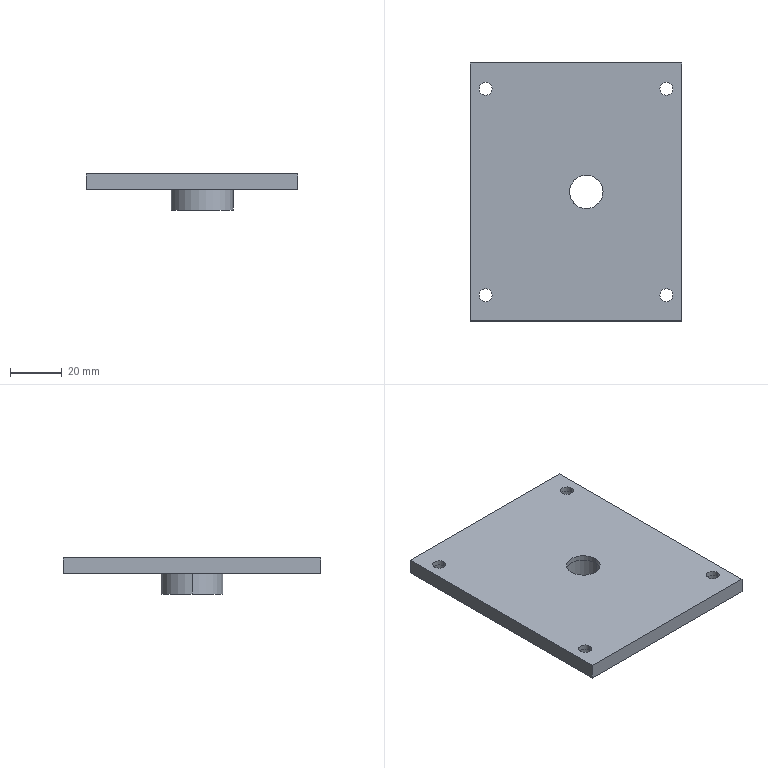Part | SolidWorks | features ICE 5, Extrusion 1 | 1 solid | 34 faces | box 82 x 100 x 14 mm | volume 49472 mm3 | cylinder 22 | plane 12 | commonest cylinder face diameters 5 x8 8 x8 13 x2 15 x2 24 x2
STEP:
#1=CARTESIAN_POINT('',(37.5,40.,6.));
#2=VERTEX_POINT('',#1);
#3=CARTESIAN_POINT('',(32.5,40.,6.));
#4=VERTEX_POINT('',#3);
#5=CARTESIAN_POINT('',(35.,40.,6.));
#6=DIRECTION('',(0.,0.,-1.));
#7=DIRECTION('',(1.,0.,0.));
#8=AXIS2_PLACEMENT_3D('',#5,#6,#7);
#9=CIRCLE('',#8,2.5);
#10=EDGE_CURVE('',#2,#4,#9,.T.);
#11=ORIENTED_EDGE('',*,*,#10,.F.);
#12=CARTESIAN_POINT('',(37.5,40.,4.));
#13=VERTEX_POINT('',#12);
#14=CARTESIAN_POINT('',(37.5,40.,6.));
#15=DIRECTION('',(0.,0.,-1.));
#16=VECTOR('',#15,1000.);
#17=LINE('',#14,#16);
#18=EDGE_CURVE('',#2,#13,#17,.T.);
#19=ORIENTED_EDGE('',*,*,#18,.T.);
#20=CARTESIAN_POINT('',(32.5,40.,4.));
#21=VERTEX_POINT('',#20);
#22=CARTESIAN_POINT('',(35.,40.,4.));
#23=DIRECTION('',(0.,0.,-1.));
#24=DIRECTION('',(-1.,0.,0.));
#25=AXIS2_PLACEMENT_3D('',#22,#23,#24);
#26=CIRCLE('',#25,2.5);
#27=EDGE_CURVE('',#13,#21,#26,.T.);
#28=ORIENTED_EDGE('',*,*,#27,.T.);
#29=CARTESIAN_POINT('',(32.5,40.,6.));
#30=DIRECTION('',(0.,0.,-1.));
#31=VECTOR('',#30,1000.);
#32=LINE('',#29,#31);
#33=EDGE_CURVE('',#4,#21,#32,.T.);
#34=ORIENTED_EDGE('',*,*,#33,.F.);
#35=EDGE_LOOP('',(#11,#19,#28,#34));
#36=FACE_OUTER_BOUND('',#35,.T.);
#37=CARTESIAN_POINT('',(35.,40.,6.));
#38=DIRECTION('',(0.,0.,-1.));
#39=DIRECTION('',(-1.,0.,0.));
#40=AXIS2_PLACEMENT_3D('',#37,#38,#39);
#41=CYLINDRICAL_SURFACE('',#40,2.5);
#42=ADVANCED_FACE('',(#36),#41,.F.);
#43=CARTESIAN_POINT('',(37.5,-40.,6.));
#44=VERTEX_POINT('',#43);
#45=CARTESIAN_POINT('',(32.5,-40.,6.));
#46=VERTEX_POINT('',#45);
#47=CARTESIAN_POINT('',(35.,-40.,6.));
#48=DIRECTION('',(0.,0.,-1.));
#49=DIRECTION('',(-1.,0.,0.));
#50=AXIS2_PLACEMENT_3D('',#47,#48,#49);
#51=CIRCLE('',#50,2.5);
#52=EDGE_CURVE('',#44,#46,#51,.T.);
#53=ORIENTED_EDGE('',*,*,#52,.F.);
#54=CARTESIAN_POINT('',(37.5,-40.,4.));
#55=VERTEX_POINT('',#54);
#56=CARTESIAN_POINT('',(37.5,-40.,6.));
#57=DIRECTION('',(0.,0.,-1.));
#58=VECTOR('',#57,1000.);
#59=LINE('',#56,#58);
#60=EDGE_CURVE('',#44,#55,#59,.T.);
#61=ORIENTED_EDGE('',*,*,#60,.T.);
#62=CARTESIAN_POINT('',(32.5,-40.,4.));
#63=VERTEX_POINT('',#62);
#64=CARTESIAN_POINT('',(35.,-40.,4.));
#65=DIRECTION('',(0.,0.,1.));
#66=DIRECTION('',(1.,0.,0.));
#67=AXIS2_PLACEMENT_3D('',#64,#65,#66);
#68=CIRCLE('',#67,2.5);
#69=EDGE_CURVE('',#63,#55,#68,.T.);
#70=ORIENTED_EDGE('',*,*,#69,.F.);
#71=CARTESIAN_POINT('',(32.5,-40.,6.));
#72=DIRECTION('',(0.,0.,-1.));
#73=VECTOR('',#72,1000.);
#74=LINE('',#71,#73);
#75=EDGE_CURVE('',#46,#63,#74,.T.);
#76=ORIENTED_EDGE('',*,*,#75,.F.);
#77=EDGE_LOOP('',(#53,#61,#70,#76));
#78=FACE_OUTER_BOUND('',#77,.T.);
#79=CARTESIAN_POINT('',(35.,-40.,6.));
#80=DIRECTION('',(0.,0.,-1.));
#81=DIRECTION('',(-1.,0.,0.));
#82=AXIS2_PLACEMENT_3D('',#79,#80,#81);
#83=CYLINDRICAL_SURFACE('',#82,2.5);
#84=ADVANCED_FACE('',(#78),#83,.F.);
#85=CARTESIAN_POINT('',(-32.5,-40.,6.));
#86=VERTEX_POINT('',#85);
#87=CARTESIAN_POINT('',(-37.5,-40.,6.));
#88=VERTEX_POINT('',#87);
#89=CARTESIAN_POINT('',(-35.,-40.,6.));
#90=DIRECTION('',(0.,0.,-1.));
#91=DIRECTION('',(1.,0.,0.));
#92=AXIS2_PLACEMENT_3D('',#89,#90,#91);
#93=CIRCLE('',#92,2.5);
#94=EDGE_CURVE('',#86,#88,#93,.T.);
#95=ORIENTED_EDGE('',*,*,#94,.F.);
#96=CARTESIAN_POINT('',(-32.5,-40.,4.));
#97=VERTEX_POINT('',#96);
#98=CARTESIAN_POINT('',(-32.5,-40.,6.));
#99=DIRECTION('',(0.,0.,-1.));
#100=VECTOR('',#99,1000.);
#101=LINE('',#98,#100);
#102=EDGE_CURVE('',#86,#97,#101,.T.);
#103=ORIENTED_EDGE('',*,*,#102,.T.);
#104=CARTESIAN_POINT('',(-37.5,-40.,4.));
#105=VERTEX_POINT('',#104);
#106=CARTESIAN_POINT('',(-35.,-40.,4.));
#107=DIRECTION('',(0.,0.,-1.));
#108=DIRECTION('',(-1.,0.,0.));
#109=AXIS2_PLACEMENT_3D('',#106,#107,#108);
#110=CIRCLE('',#109,2.5);
#111=EDGE_CURVE('',#97,#105,#110,.T.);
#112=ORIENTED_EDGE('',*,*,#111,.T.);
#113=CARTESIAN_POINT('',(-37.5,-40.,6.));
#114=DIRECTION('',(0.,0.,-1.));
#115=VECTOR('',#114,1000.);
#116=LINE('',#113,#115);
#117=EDGE_CURVE('',#88,#105,#116,.T.);
#118=ORIENTED_EDGE('',*,*,#117,.F.);
#119=EDGE_LOOP('',(#95,#103,#112,#118));
#120=FACE_OUTER_BOUND('',#119,.T.);
#121=CARTESIAN_POINT('',(-35.,-40.,6.));
#122=DIRECTION('',(0.,0.,-1.));
#123=DIRECTION('',(-1.,0.,0.));
#124=AXIS2_PLACEMENT_3D('',#121,#122,#123);
#125=CYLINDRICAL_SURFACE('',#124,2.5);
#126=ADVANCED_FACE('',(#120),#125,.F.);
#127=CARTESIAN_POINT('',(-32.5,40.,6.));
#128=VERTEX_POINT('',#127);
#129=CARTESIAN_POINT('',(-37.5,40.,6.));
#130=VERTEX_POINT('',#129);
#131=CARTESIAN_POINT('',(-35.,40.,6.));
#132=DIRECTION('',(0.,0.,-1.));
#133=DIRECTION('',(-1.,0.,0.));
#134=AXIS2_PLACEMENT_3D('',#131,#132,#133);
#135=CIRCLE('',#134,2.5);
#136=EDGE_CURVE('',#128,#130,#135,.T.);
#137=ORIENTED_EDGE('',*,*,#136,.F.);
#138=CARTESIAN_POINT('',(-32.5,40.,4.));
#139=VERTEX_POINT('',#138);
#140=CARTESIAN_POINT('',(-32.5,40.,6.));
#141=DIRECTION('',(0.,0.,-1.));
#142=VECTOR('',#141,1000.);
#143=LINE('',#140,#142);
#144=EDGE_CURVE('',#128,#139,#143,.T.);
#145=ORIENTED_EDGE('',*,*,#144,.T.);
#146=CARTESIAN_POINT('',(-37.5,40.,4.));
#147=VERTEX_POINT('',#146);
#148=CARTESIAN_POINT('',(-35.,40.,4.));
#149=DIRECTION('',(0.,0.,1.));
#150=DIRECTION('',(1.,0.,0.));
#151=AXIS2_PLACEMENT_3D('',#148,#149,#150);
#152=CIRCLE('',#151,2.5);
#153=EDGE_CURVE('',#147,#139,#152,.T.);
#154=ORIENTED_EDGE('',*,*,#153,.F.);
#155=CARTESIAN_POINT('',(-37.5,40.,6.));
#156=DIRECTION('',(0.,0.,-1.));
#157=VECTOR('',#156,1000.);
#158=LINE('',#155,#157);
#159=EDGE_CURVE('',#130,#147,#158,.T.);
#160=ORIENTED_EDGE('',*,*,#159,.F.);
#161=EDGE_LOOP('',(#137,#145,#154,#160));
#162=FACE_OUTER_BOUND('',#161,.T.);
#163=CARTESIAN_POINT('',(-35.,40.,6.));
#164=DIRECTION('',(0.,0.,-1.));
#165=DIRECTION('',(-1.,0.,0.));
#166=AXIS2_PLACEMENT_3D('',#163,#164,#165);
#167=CYLINDRICAL_SURFACE('',#166,2.5);
#168=ADVANCED_FACE('',(#162),#167,.F.);
#169=CARTESIAN_POINT('',(11.5,0.,4.));
#170=VERTEX_POINT('',#169);
#171=CARTESIAN_POINT('',(-3.5,0.,4.));
#172=VERTEX_POINT('',#171);
#173=CARTESIAN_POINT('',(4.,0.,4.));
#174=DIRECTION('',(0.,0.,-1.));
#175=DIRECTION('',(-1.,0.,0.));
#176=AXIS2_PLACEMENT_3D('',#173,#174,#175);
#177=CIRCLE('',#176,7.5);
#178=EDGE_CURVE('',#170,#172,#177,.T.);
#179=ORIENTED_EDGE('',*,*,#178,.F.);
#180=CARTESIAN_POINT('',(11.5,0.,-8.));
#181=VERTEX_POINT('',#180);
#182=CARTESIAN_POINT('',(11.5,0.,4.));
#183=DIRECTION('',(0.,0.,-1.));
#184=VECTOR('',#183,1000.);
#185=LINE('',#182,#184);
#186=EDGE_CURVE('',#170,#181,#185,.T.);
#187=ORIENTED_EDGE('',*,*,#186,.T.);
#188=CARTESIAN_POINT('',(-3.5,0.,-8.));
#189=VERTEX_POINT('',#188);
#190=CARTESIAN_POINT('',(4.,0.,-8.));
#191=DIRECTION('',(0.,0.,-1.));
#192=DIRECTION('',(-1.,0.,0.));
#193=AXIS2_PLACEMENT_3D('',#190,#191,#192);
#194=CIRCLE('',#193,7.5);
#195=EDGE_CURVE('',#181,#189,#194,.T.);
#196=ORIENTED_EDGE('',*,*,#195,.T.);
#197=CARTESIAN_POINT('',(-3.5,0.,4.));
#198=DIRECTION('',(0.,0.,-1.));
#199=VECTOR('',#198,1000.);
#200=LINE('',#197,#199);
#201=EDGE_CURVE('',#172,#189,#200,.T.);
#202=ORIENTED_EDGE('',*,*,#201,.F.);
#203=EDGE_LOOP('',(#179,#187,#196,#202));
#204=FACE_OUTER_BOUND('',#203,.T.);
#205=CARTESIAN_POINT('',(4.,0.,4.));
#206=DIRECTION('',(0.,0.,-1.));
#207=DIRECTION('',(-1.,0.,0.));
#208=AXIS2_PLACEMENT_3D('',#205,#206,#207);
#209=CYLINDRICAL_SURFACE('',#208,7.5);
#210=ADVANCED_FACE('',(#204),#209,.F.);
#211=CARTESIAN_POINT('',(-2.5,0.,4.));
#212=VERTEX_POINT('',#211);
#213=CARTESIAN_POINT('',(10.5,0.,4.));
#214=VERTEX_POINT('',#213);
#215=CARTESIAN_POINT('',(4.,0.,4.));
#216=DIRECTION('',(0.,0.,1.));
#217=DIRECTION('',(1.,0.,0.));
#218=AXIS2_PLACEMENT_3D('',#215,#216,#217);
#219=CIRCLE('',#218,6.5);
#220=EDGE_CURVE('',#212,#214,#219,.T.);
#221=ORIENTED_EDGE('',*,*,#220,.F.);
#222=CARTESIAN_POINT('',(-2.5,0.,6.));
#223=VERTEX_POINT('',#222);
#224=CARTESIAN_POINT('',(-2.5,0.,4.));
#225=DIRECTION('',(0.,0.,1.));
#226=VECTOR('',#225,1000.);
#227=LINE('',#224,#226);
#228=EDGE_CURVE('',#212,#223,#227,.T.);
#229=ORIENTED_EDGE('',*,*,#228,.T.);
#230=CARTESIAN_POINT('',(10.5,0.,6.));
#231=VERTEX_POINT('',#230);
#232=CARTESIAN_POINT('',(4.,0.,6.));
#233=DIRECTION('',(0.,0.,1.));
#234=DIRECTION('',(1.,0.,0.));
#235=AXIS2_PLACEMENT_3D('',#232,#233,#234);
#236=CIRCLE('',#235,6.5);
#237=EDGE_CURVE('',#223,#231,#236,.T.);
#238=ORIENTED_EDGE('',*,*,#237,.T.);
#239=CARTESIAN_POINT('',(10.5,0.,4.));
#240=DIRECTION('',(0.,0.,1.));
#241=VECTOR('',#240,1000.);
#242=LINE('',#239,#241);
#243=EDGE_CURVE('',#214,#231,#242,.T.);
#244=ORIENTED_EDGE('',*,*,#243,.F.);
#245=EDGE_LOOP('',(#221,#229,#238,#244));
#246=FACE_OUTER_BOUND('',#245,.T.);
#247=CARTESIAN_POINT('',(4.,0.,4.));
#248=DIRECTION('',(0.,0.,1.));
#249=DIRECTION('',(1.,0.,0.));
#250=AXIS2_PLACEMENT_3D('',#247,#248,#249);
#251=CYLINDRICAL_SURFACE('',#250,6.5);
#252=ADVANCED_FACE('',(#246),#251,.F.);
#253=CARTESIAN_POINT('',(-31.,40.,4.));
#254=VERTEX_POINT('',#253);
#255=CARTESIAN_POINT('',(-39.,40.,4.));
#256=VERTEX_POINT('',#255);
#257=CARTESIAN_POINT('',(-35.,40.,4.));
#258=DIRECTION('',(0.,0.,-1.));
#259=DIRECTION('',(1.,0.,0.));
#260=AXIS2_PLACEMENT_3D('',#257,#258,#259);
#261=CIRCLE('',#260,4.);
#262=EDGE_CURVE('',#254,#256,#261,.T.);
#263=ORIENTED_EDGE('',*,*,#262,.F.);
#264=CARTESIAN_POINT('',(-31.,40.,0.));
#265=VERTEX_POINT('',#264);
#266=CARTESIAN_POINT('',(-31.,40.,4.));
#267=DIRECTION('',(0.,0.,-1.));
#268=VECTOR('',#267,1000.);
#269=LINE('',#266,#268);
#270=EDGE_CURVE('',#254,#265,#269,.T.);
#271=ORIENTED_EDGE('',*,*,#270,.T.);
#272=CARTESIAN_POINT('',(-39.,40.,0.));
#273=VERTEX_POINT('',#272);
#274=CARTESIAN_POINT('',(-35.,40.,0.));
#275=DIRECTION('',(0.,0.,-1.));
#276=DIRECTION('',(1.,0.,0.));
#277=AXIS2_PLACEMENT_3D('',#274,#275,#276);
#278=CIRCLE('',#277,4.);
#279=EDGE_CURVE('',#265,#273,#278,.T.);
#280=ORIENTED_EDGE('',*,*,#279,.T.);
#281=CARTESIAN_POINT('',(-39.,40.,4.));
#282=DIRECTION('',(0.,0.,-1.));
#283=VECTOR('',#282,1000.);
#284=LINE('',#281,#283);
#285=EDGE_CURVE('',#256,#273,#284,.T.);
#286=ORIENTED_EDGE('',*,*,#285,.F.);
#287=EDGE_LOOP('',(#263,#271,#280,#286));
#288=FACE_OUTER_BOUND('',#287,.T.);
#289=CARTESIAN_POINT('',(-35.,40.,4.));
#290=DIRECTION('',(0.,0.,-1.));
#291=DIRECTION('',(-1.,0.,0.));
#292=AXIS2_PLACEMENT_3D('',#289,#290,#291);
#293=CYLINDRICAL_SURFACE('',#292,4.);
#294=ADVANCED_FACE('',(#288),#293,.F.);
#295=CARTESIAN_POINT('',(-31.,-40.,4.));
#296=VERTEX_POINT('',#295);
#297=CARTESIAN_POINT('',(-39.,-40.,4.));
#298=VERTEX_POINT('',#297);
#299=CARTESIAN_POINT('',(-35.,-40.,4.));
#300=DIRECTION('',(0.,0.,-1.));
#301=DIRECTION('',(-1.,0.,0.));
#302=AXIS2_PLACEMENT_3D('',#299,#300,#301);
#303=CIRCLE('',#302,4.);
#304=EDGE_CURVE('',#296,#298,#303,.T.);
#305=ORIENTED_EDGE('',*,*,#304,.F.);
#306=CARTESIAN_POINT('',(-31.,-40.,0.));
#307=VERTEX_POINT('',#306);
#308=CARTESIAN_POINT('',(-31.,-40.,4.));
#309=DIRECTION('',(0.,0.,-1.));
#310=VECTOR('',#309,1000.);
#311=LINE('',#308,#310);
#312=EDGE_CURVE('',#296,#307,#311,.T.);
#313=ORIENTED_EDGE('',*,*,#312,.T.);
#314=CARTESIAN_POINT('',(-39.,-40.,0.));
#315=VERTEX_POINT('',#314);
#316=CARTESIAN_POINT('',(-35.,-40.,0.));
#317=DIRECTION('',(0.,0.,-1.));
#318=DIRECTION('',(-1.,0.,0.));
#319=AXIS2_PLACEMENT_3D('',#316,#317,#318);
#320=CIRCLE('',#319,4.);
#321=EDGE_CURVE('',#307,#315,#320,.T.);
#322=ORIENTED_EDGE('',*,*,#321,.T.);
#323=CARTESIAN_POINT('',(-39.,-40.,4.));
#324=DIRECTION('',(0.,0.,-1.));
#325=VECTOR('',#324,1000.);
#326=LINE('',#323,#325);
#327=EDGE_CURVE('',#298,#315,#326,.T.);
#328=ORIENTED_EDGE('',*,*,#327,.F.);
#329=EDGE_LOOP('',(#305,#313,#322,#328));
#330=FACE_OUTER_BOUND('',#329,.T.);
#331=CARTESIAN_POINT('',(-35.,-40.,4.));
#332=DIRECTION('',(0.,0.,-1.));
#333=DIRECTION('',(-1.,0.,0.));
#334=AXIS2_PLACEMENT_3D('',#331,#332,#333);
#335=CYLINDRICAL_SURFACE('',#334,4.);
#336=ADVANCED_FACE('',(#330),#335,.F.);
#337=CARTESIAN_POINT('',(39.,-40.,4.));
#338=VERTEX_POINT('',#337);
#339=CARTESIAN_POINT('',(31.,-40.,4.));
#340=VERTEX_POINT('',#339);
#341=CARTESIAN_POINT('',(35.,-40.,4.));
#342=DIRECTION('',(0.,0.,-1.));
#343=DIRECTION('',(1.,0.,0.));
#344=AXIS2_PLACEMENT_3D('',#341,#342,#343);
#345=CIRCLE('',#344,4.);
#346=EDGE_CURVE('',#338,#340,#345,.T.);
#347=ORIENTED_EDGE('',*,*,#346,.F.);
#348=CARTESIAN_POINT('',(39.,-40.,0.));
#349=VERTEX_POINT('',#348);
#350=CARTESIAN_POINT('',(39.,-40.,4.));
#351=DIRECTION('',(0.,0.,-1.));
#352=VECTOR('',#351,1000.);
#353=LINE('',#350,#352);
#354=EDGE_CURVE('',#338,#349,#353,.T.);
#355=ORIENTED_EDGE('',*,*,#354,.T.);
#356=CARTESIAN_POINT('',(31.,-40.,0.));
#357=VERTEX_POINT('',#356);
#358=CARTESIAN_POINT('',(35.,-40.,0.));
#359=DIRECTION('',(0.,0.,-1.));
#360=DIRECTION('',(1.,0.,0.));
#361=AXIS2_PLACEMENT_3D('',#358,#359,#360);
#362=CIRCLE('',#361,4.);
#363=EDGE_CURVE('',#349,#357,#362,.T.);
#364=ORIENTED_EDGE('',*,*,#363,.T.);
#365=CARTESIAN_POINT('',(31.,-40.,4.));
#366=DIRECTION('',(0.,0.,-1.));
#367=VECTOR('',#366,1000.);
#368=LINE('',#365,#367);
#369=EDGE_CURVE('',#340,#357,#368,.T.);
#370=ORIENTED_EDGE('',*,*,#369,.F.);
#371=EDGE_LOOP('',(#347,#355,#364,#370));
#372=FACE_OUTER_BOUND('',#371,.T.);
#373=CARTESIAN_POINT('',(35.,-40.,4.));
#374=DIRECTION('',(0.,0.,-1.));
#375=DIRECTION('',(-1.,0.,0.));
#376=AXIS2_PLACEMENT_3D('',#373,#374,#375);
#377=CYLINDRICAL_SURFACE('',#376,4.);
#378=ADVANCED_FACE('',(#372),#377,.F.);
#379=CARTESIAN_POINT('',(39.,40.,4.));
#380=VERTEX_POINT('',#379);
#381=CARTESIAN_POINT('',(31.,40.,4.));
#382=VERTEX_POINT('',#381);
#383=CARTESIAN_POINT('',(35.,40.,4.));
#384=DIRECTION('',(0.,0.,-1.));
#385=DIRECTION('',(-1.,0.,0.));
#386=AXIS2_PLACEMENT_3D('',#383,#384,#385);
#387=CIRCLE('',#386,4.);
#388=EDGE_CURVE('',#380,#382,#387,.T.);
#389=ORIENTED_EDGE('',*,*,#388,.F.);
#390=CARTESIAN_POINT('',(39.,40.,0.));
#391=VERTEX_POINT('',#390);
#392=CARTESIAN_POINT('',(39.,40.,4.));
#393=DIRECTION('',(0.,0.,-1.));
#394=VECTOR('',#393,1000.);
#395=LINE('',#392,#394);
#396=EDGE_CURVE('',#380,#391,#395,.T.);
#397=ORIENTED_EDGE('',*,*,#396,.T.);
#398=CARTESIAN_POINT('',(31.,40.,0.));
#399=VERTEX_POINT('',#398);
#400=CARTESIAN_POINT('',(35.,40.,0.));
#401=DIRECTION('',(0.,0.,-1.));
#402=DIRECTION('',(-1.,0.,0.));
#403=AXIS2_PLACEMENT_3D('',#400,#401,#402);
#404=CIRCLE('',#403,4.);
#405=EDGE_CURVE('',#391,#399,#404,.T.);
#406=ORIENTED_EDGE('',*,*,#405,.T.);
#407=CARTESIAN_POINT('',(31.,40.,4.));
#408=DIRECTION('',(0.,0.,-1.));
#409=VECTOR('',#408,1000.);
#410=LINE('',#407,#409);
#411=EDGE_CURVE('',#382,#399,#410,.T.);
#412=ORIENTED_EDGE('',*,*,#411,.F.);
#413=EDGE_LOOP('',(#389,#397,#406,#412));
#414=FACE_OUTER_BOUND('',#413,.T.);
#415=CARTESIAN_POINT('',(35.,40.,4.));
#416=DIRECTION('',(0.,0.,-1.));
#417=DIRECTION('',(-1.,0.,0.));
#418=AXIS2_PLACEMENT_3D('',#415,#416,#417);
#419=CYLINDRICAL_SURFACE('',#418,4.);
#420=ADVANCED_FACE('',(#414),#419,.F.);
#421=CARTESIAN_POINT('',(16.,0.,-8.));
#422=VERTEX_POINT('',#421);
#423=CARTESIAN_POINT('',(-8.,0.,-8.));
#424=VERTEX_POINT('',#423);
#425=CARTESIAN_POINT('',(4.,0.,-8.));
#426=DIRECTION('',(0.,0.,1.));
#427=DIRECTION('',(1.,0.,0.));
#428=AXIS2_PLACEMENT_3D('',#425,#426,#427);
#429=CIRCLE('',#428,12.);
#430=EDGE_CURVE('',#422,#424,#429,.T.);
#431=ORIENTED_EDGE('',*,*,#430,.T.);
#432=CARTESIAN_POINT('',(-8.,0.,0.));
#433=VERTEX_POINT('',#432);
#434=CARTESIAN_POINT('',(-8.,0.,-8.));
#435=DIRECTION('',(0.,0.,1.));
#436=VECTOR('',#435,1000.);
#437=LINE('',#434,#436);
#438=EDGE_CURVE('',#424,#433,#437,.T.);
#439=ORIENTED_EDGE('',*,*,#438,.T.);
#440=CARTESIAN_POINT('',(16.,0.,0.));
#441=VERTEX_POINT('',#440);
#442=CARTESIAN_POINT('',(4.,0.,0.));
#443=DIRECTION('',(0.,0.,1.));
#444=DIRECTION('',(1.,0.,0.));
#445=AXIS2_PLACEMENT_3D('',#442,#443,#444);
#446=CIRCLE('',#445,12.);
#447=EDGE_CURVE('',#441,#433,#446,.T.);
#448=ORIENTED_EDGE('',*,*,#447,.F.);
#449=CARTESIAN_POINT('',(16.,0.,-8.));
#450=DIRECTION('',(0.,0.,1.));
#451=VECTOR('',#450,1000.);
#452=LINE('',#449,#451);
#453=EDGE_CURVE('',#422,#441,#452,.T.);
#454=ORIENTED_EDGE('',*,*,#453,.F.);
#455=EDGE_LOOP('',(#431,#439,#448,#454));
#456=FACE_OUTER_BOUND('',#455,.T.);
#457=CARTESIAN_POINT('',(4.,0.,-8.));
#458=DIRECTION('',(0.,0.,1.));
#459=DIRECTION('',(1.,0.,0.));
#460=AXIS2_PLACEMENT_3D('',#457,#458,#459);
#461=CYLINDRICAL_SURFACE('',#460,12.);
#462=ADVANCED_FACE('',(#456),#461,.T.);
#463=CARTESIAN_POINT('',(-41.,-50.,0.));
#464=VERTEX_POINT('',#463);
#465=CARTESIAN_POINT('',(41.,-50.,0.));
#466=VERTEX_POINT('',#465);
#467=CARTESIAN_POINT('',(41.,-50.,0.));
#468=DIRECTION('',(1.,0.,0.));
#469=VECTOR('',#468,1000.);
#470=LINE('',#467,#469);
#471=EDGE_CURVE('',#464,#466,#470,.T.);
#472=ORIENTED_EDGE('',*,*,#471,.T.);
#473=CARTESIAN_POINT('',(41.,-50.,6.));
#474=VERTEX_POINT('',#473);
#475=CARTESIAN_POINT('',(41.,-50.,6.));
#476=DIRECTION('',(0.,0.,-1.));
#477=VECTOR('',#476,1000.);
#478=LINE('',#475,#477);
#479=EDGE_CURVE('',#474,#466,#478,.T.);
#480=ORIENTED_EDGE('',*,*,#479,.F.);
#481=CARTESIAN_POINT('',(-41.,-50.,6.));
#482=VERTEX_POINT('',#481);
#483=CARTESIAN_POINT('',(41.,-50.,6.));
#484=DIRECTION('',(1.,0.,0.));
#485=VECTOR('',#484,1000.);
#486=LINE('',#483,#485);
#487=EDGE_CURVE('',#482,#474,#486,.T.);
#488=ORIENTED_EDGE('',*,*,#487,.F.);
#489=CARTESIAN_POINT('',(-41.,-50.,6.));
#490=DIRECTION('',(0.,0.,-1.));
#491=VECTOR('',#490,1000.);
#492=LINE('',#489,#491);
#493=EDGE_CURVE('',#482,#464,#492,.T.);
#494=ORIENTED_EDGE('',*,*,#493,.T.);
#495=EDGE_LOOP('',(#472,#480,#488,#494));
#496=FACE_OUTER_BOUND('',#495,.T.);
#497=CARTESIAN_POINT('',(41.,-50.,6.));
#498=DIRECTION('',(0.,1.,0.));
#499=DIRECTION('',(-1.,0.,0.));
#500=AXIS2_PLACEMENT_3D('',#497,#498,#499);
#501=PLANE('',#500);
#502=ADVANCED_FACE('',(#496),#501,.F.);
#503=CARTESIAN_POINT('',(41.,50.,0.));
#504=VERTEX_POINT('',#503);
#505=CARTESIAN_POINT('',(41.,50.,0.));
#506=DIRECTION('',(0.,1.,0.));
#507=VECTOR('',#506,1000.);
#508=LINE('',#505,#507);
#509=EDGE_CURVE('',#466,#504,#508,.T.);
#510=ORIENTED_EDGE('',*,*,#509,.T.);
#511=CARTESIAN_POINT('',(41.,50.,6.));
#512=VERTEX_POINT('',#511);
#513=CARTESIAN_POINT('',(41.,50.,6.));
#514=DIRECTION('',(0.,0.,-1.));
#515=VECTOR('',#514,1000.);
#516=LINE('',#513,#515);
#517=EDGE_CURVE('',#512,#504,#516,.T.);
#518=ORIENTED_EDGE('',*,*,#517,.F.);
#519=CARTESIAN_POINT('',(41.,50.,6.));
#520=DIRECTION('',(0.,1.,0.));
#521=VECTOR('',#520,1000.);
#522=LINE('',#519,#521);
#523=EDGE_CURVE('',#474,#512,#522,.T.);
#524=ORIENTED_EDGE('',*,*,#523,.F.);
#525=ORIENTED_EDGE('',*,*,#479,.T.);
#526=EDGE_LOOP('',(#510,#518,#524,#525));
#527=FACE_OUTER_BOUND('',#526,.T.);
#528=CARTESIAN_POINT('',(41.,50.,6.));
#529=DIRECTION('',(-1.,0.,0.));
#530=DIRECTION('',(0.,0.,1.));
#531=AXIS2_PLACEMENT_3D('',#528,#529,#530);
#532=PLANE('',#531);
#533=ADVANCED_FACE('',(#527),#532,.F.);
#534=CARTESIAN_POINT('',(-41.,50.,0.));
#535=VERTEX_POINT('',#534);
#536=CARTESIAN_POINT('',(41.,50.,0.));
#537=DIRECTION('',(-1.,0.,0.));
#538=VECTOR('',#537,1000.);
#539=LINE('',#536,#538);
#540=EDGE_CURVE('',#504,#535,#539,.T.);
#541=ORIENTED_EDGE('',*,*,#540,.T.);
#542=CARTESIAN_POINT('',(-41.,50.,6.));
#543=VERTEX_POINT('',#542);
#544=CARTESIAN_POINT('',(-41.,50.,6.));
#545=DIRECTION('',(0.,0.,-1.));
#546=VECTOR('',#545,1000.);
#547=LINE('',#544,#546);
#548=EDGE_CURVE('',#543,#535,#547,.T.);
#549=ORIENTED_EDGE('',*,*,#548,.F.);
#550=CARTESIAN_POINT('',(41.,50.,6.));
#551=DIRECTION('',(-1.,0.,0.));
#552=VECTOR('',#551,1000.);
#553=LINE('',#550,#552);
#554=EDGE_CURVE('',#512,#543,#553,.T.);
#555=ORIENTED_EDGE('',*,*,#554,.F.);
#556=ORIENTED_EDGE('',*,*,#517,.T.);
#557=EDGE_LOOP('',(#541,#549,#555,#556));
#558=FACE_OUTER_BOUND('',#557,.T.);
#559=CARTESIAN_POINT('',(41.,50.,6.));
#560=DIRECTION('',(0.,-1.,0.));
#561=DIRECTION('',(1.,0.,0.));
#562=AXIS2_PLACEMENT_3D('',#559,#560,#561);
#563=PLANE('',#562);
#564=ADVANCED_FACE('',(#558),#563,.F.);
#565=CARTESIAN_POINT('',(-41.,50.,0.));
#566=DIRECTION('',(0.,-1.,0.));
#567=VECTOR('',#566,1000.);
#568=LINE('',#565,#567);
#569=EDGE_CURVE('',#535,#464,#568,.T.);
#570=ORIENTED_EDGE('',*,*,#569,.T.);
#571=ORIENTED_EDGE('',*,*,#493,.F.);
#572=CARTESIAN_POINT('',(-41.,50.,6.));
#573=DIRECTION('',(0.,-1.,0.));
#574=VECTOR('',#573,1000.);
#575=LINE('',#572,#574);
#576=EDGE_CURVE('',#543,#482,#575,.T.);
#577=ORIENTED_EDGE('',*,*,#576,.F.);
#578=ORIENTED_EDGE('',*,*,#548,.T.);
#579=EDGE_LOOP('',(#570,#571,#577,#578));
#580=FACE_OUTER_BOUND('',#579,.T.);
#581=CARTESIAN_POINT('',(-41.,50.,6.));
#582=DIRECTION('',(1.,0.,0.));
#583=DIRECTION('',(0.,0.,-1.));
#584=AXIS2_PLACEMENT_3D('',#581,#582,#583);
#585=PLANE('',#584);
#586=ADVANCED_FACE('',(#580),#585,.F.);
#587=CARTESIAN_POINT('',(35.,40.,6.));
#588=DIRECTION('',(0.,0.,-1.));
#589=DIRECTION('',(1.,0.,0.));
#590=AXIS2_PLACEMENT_3D('',#587,#588,#589);
#591=CIRCLE('',#590,2.5);
#592=EDGE_CURVE('',#4,#2,#591,.T.);
#593=ORIENTED_EDGE('',*,*,#592,.T.);
#594=ORIENTED_EDGE('',*,*,#10,.T.);
#595=EDGE_LOOP('',(#593,#594));
#596=FACE_BOUND('',#595,.T.);
#597=CARTESIAN_POINT('',(-35.,-40.,6.));
#598=DIRECTION('',(0.,0.,-1.));
#599=DIRECTION('',(1.,0.,0.));
#600=AXIS2_PLACEMENT_3D('',#597,#598,#599);
#601=CIRCLE('',#600,2.5);
#602=EDGE_CURVE('',#88,#86,#601,.T.);
#603=ORIENTED_EDGE('',*,*,#602,.T.);
#604=ORIENTED_EDGE('',*,*,#94,.T.);
#605=EDGE_LOOP('',(#603,#604));
#606=FACE_BOUND('',#605,.T.);
#607=CARTESIAN_POINT('',(-35.,40.,6.));
#608=DIRECTION('',(0.,0.,-1.));
#609=DIRECTION('',(-1.,0.,0.));
#610=AXIS2_PLACEMENT_3D('',#607,#608,#609);
#611=CIRCLE('',#610,2.5);
#612=EDGE_CURVE('',#130,#128,#611,.T.);
#613=ORIENTED_EDGE('',*,*,#612,.T.);
#614=ORIENTED_EDGE('',*,*,#136,.T.);
#615=EDGE_LOOP('',(#613,#614));
#616=FACE_BOUND('',#615,.T.);
#617=CARTESIAN_POINT('',(35.,-40.,6.));
#618=DIRECTION('',(0.,0.,-1.));
#619=DIRECTION('',(-1.,0.,0.));
#620=AXIS2_PLACEMENT_3D('',#617,#618,#619);
#621=CIRCLE('',#620,2.5);
#622=EDGE_CURVE('',#46,#44,#621,.T.);
#623=ORIENTED_EDGE('',*,*,#622,.T.);
#624=ORIENTED_EDGE('',*,*,#52,.T.);
#625=EDGE_LOOP('',(#623,#624));
#626=FACE_BOUND('',#625,.T.);
#627=CARTESIAN_POINT('',(4.,0.,6.));
#628=DIRECTION('',(0.,0.,1.));
#629=DIRECTION('',(1.,0.,0.));
#630=AXIS2_PLACEMENT_3D('',#627,#628,#629);
#631=CIRCLE('',#630,6.5);
#632=EDGE_CURVE('',#231,#223,#631,.T.);
#633=ORIENTED_EDGE('',*,*,#632,.F.);
#634=ORIENTED_EDGE('',*,*,#237,.F.);
#635=EDGE_LOOP('',(#633,#634));
#636=FACE_BOUND('',#635,.T.);
#637=ORIENTED_EDGE('',*,*,#487,.T.);
#638=ORIENTED_EDGE('',*,*,#523,.T.);
#639=ORIENTED_EDGE('',*,*,#554,.T.);
#640=ORIENTED_EDGE('',*,*,#576,.T.);
#641=EDGE_LOOP('',(#637,#638,#639,#640));
#642=FACE_OUTER_BOUND('',#641,.T.);
#643=CARTESIAN_POINT('',(0.,0.,6.));
#644=DIRECTION('',(0.,0.,1.));
#645=DIRECTION('',(1.,0.,0.));
#646=AXIS2_PLACEMENT_3D('',#643,#644,#645);
#647=PLANE('',#646);
#648=ADVANCED_FACE('',(#596,#606,#616,#626,#636,#642),#647,.T.);
#649=CARTESIAN_POINT('',(-35.,40.,0.));
#650=DIRECTION('',(0.,0.,-1.));
#651=DIRECTION('',(1.,0.,0.));
#652=AXIS2_PLACEMENT_3D('',#649,#650,#651);
#653=CIRCLE('',#652,4.);
#654=EDGE_CURVE('',#273,#265,#653,.T.);
#655=ORIENTED_EDGE('',*,*,#654,.F.);
#656=ORIENTED_EDGE('',*,*,#279,.F.);
#657=EDGE_LOOP('',(#655,#656));
#658=FACE_BOUND('',#657,.T.);
#659=CARTESIAN_POINT('',(-35.,-40.,0.));
#660=DIRECTION('',(0.,0.,-1.));
#661=DIRECTION('',(-1.,0.,0.));
#662=AXIS2_PLACEMENT_3D('',#659,#660,#661);
#663=CIRCLE('',#662,4.);
#664=EDGE_CURVE('',#315,#307,#663,.T.);
#665=ORIENTED_EDGE('',*,*,#664,.F.);
#666=ORIENTED_EDGE('',*,*,#321,.F.);
#667=EDGE_LOOP('',(#665,#666));
#668=FACE_BOUND('',#667,.T.);
#669=CARTESIAN_POINT('',(35.,-40.,0.));
#670=DIRECTION('',(0.,0.,-1.));
#671=DIRECTION('',(1.,0.,0.));
#672=AXIS2_PLACEMENT_3D('',#669,#670,#671);
#673=CIRCLE('',#672,4.);
#674=EDGE_CURVE('',#357,#349,#673,.T.);
#675=ORIENTED_EDGE('',*,*,#674,.F.);
#676=ORIENTED_EDGE('',*,*,#363,.F.);
#677=EDGE_LOOP('',(#675,#676));
#678=FACE_BOUND('',#677,.T.);
#679=CARTESIAN_POINT('',(35.,40.,0.));
#680=DIRECTION('',(0.,0.,-1.));
#681=DIRECTION('',(-1.,0.,0.));
#682=AXIS2_PLACEMENT_3D('',#679,#680,#681);
#683=CIRCLE('',#682,4.);
#684=EDGE_CURVE('',#399,#391,#683,.T.);
#685=ORIENTED_EDGE('',*,*,#684,.F.);
#686=ORIENTED_EDGE('',*,*,#405,.F.);
#687=EDGE_LOOP('',(#685,#686));
#688=FACE_BOUND('',#687,.T.);
#689=ORIENTED_EDGE('',*,*,#447,.T.);
#690=CARTESIAN_POINT('',(4.,0.,0.));
#691=DIRECTION('',(0.,0.,1.));
#692=DIRECTION('',(1.,0.,0.));
#693=AXIS2_PLACEMENT_3D('',#690,#691,#692);
#694=CIRCLE('',#693,12.);
#695=EDGE_CURVE('',#433,#441,#694,.T.);
#696=ORIENTED_EDGE('',*,*,#695,.T.);
#697=EDGE_LOOP('',(#689,#696));
#698=FACE_BOUND('',#697,.T.);
#699=ORIENTED_EDGE('',*,*,#471,.F.);
#700=ORIENTED_EDGE('',*,*,#569,.F.);
#701=ORIENTED_EDGE('',*,*,#540,.F.);
#702=ORIENTED_EDGE('',*,*,#509,.F.);
#703=EDGE_LOOP('',(#699,#700,#701,#702));
#704=FACE_OUTER_BOUND('',#703,.T.);
#705=CARTESIAN_POINT('',(0.,0.,0.));
#706=DIRECTION('',(0.,0.,1.));
#707=DIRECTION('',(1.,0.,0.));
#708=AXIS2_PLACEMENT_3D('',#705,#706,#707);
#709=PLANE('',#708);
#710=ADVANCED_FACE('',(#658,#668,#678,#688,#698,#704),#709,.F.);
#711=ORIENTED_EDGE('',*,*,#438,.F.);
#712=CARTESIAN_POINT('',(4.,0.,-8.));
#713=DIRECTION('',(0.,0.,1.));
#714=DIRECTION('',(1.,0.,0.));
#715=AXIS2_PLACEMENT_3D('',#712,#713,#714);
#716=CIRCLE('',#715,12.);
#717=EDGE_CURVE('',#424,#422,#716,.T.);
#718=ORIENTED_EDGE('',*,*,#717,.T.);
#719=ORIENTED_EDGE('',*,*,#453,.T.);
#720=ORIENTED_EDGE('',*,*,#695,.F.);
#721=EDGE_LOOP('',(#711,#718,#719,#720));
#722=FACE_OUTER_BOUND('',#721,.T.);
#723=CARTESIAN_POINT('',(4.,0.,-8.));
#724=DIRECTION('',(0.,0.,1.));
#725=DIRECTION('',(1.,0.,0.));
#726=AXIS2_PLACEMENT_3D('',#723,#724,#725);
#727=CYLINDRICAL_SURFACE('',#726,12.);
#728=ADVANCED_FACE('',(#722),#727,.T.);
#729=CARTESIAN_POINT('',(4.,0.,-8.));
#730=DIRECTION('',(0.,0.,-1.));
#731=DIRECTION('',(-1.,0.,0.));
#732=AXIS2_PLACEMENT_3D('',#729,#730,#731);
#733=CIRCLE('',#732,7.5);
#734=EDGE_CURVE('',#189,#181,#733,.T.);
#735=ORIENTED_EDGE('',*,*,#734,.F.);
#736=ORIENTED_EDGE('',*,*,#195,.F.);
#737=EDGE_LOOP('',(#735,#736));
#738=FACE_BOUND('',#737,.T.);
#739=ORIENTED_EDGE('',*,*,#430,.F.);
#740=ORIENTED_EDGE('',*,*,#717,.F.);
#741=EDGE_LOOP('',(#739,#740));
#742=FACE_OUTER_BOUND('',#741,.T.);
#743=CARTESIAN_POINT('',(4.,0.,-8.));
#744=DIRECTION('',(0.,0.,1.));
#745=DIRECTION('',(1.,0.,0.));
#746=AXIS2_PLACEMENT_3D('',#743,#744,#745);
#747=PLANE('',#746);
#748=ADVANCED_FACE('',(#738,#742),#747,.F.);
#749=ORIENTED_EDGE('',*,*,#396,.F.);
#750=CARTESIAN_POINT('',(35.,40.,4.));
#751=DIRECTION('',(0.,0.,-1.));
#752=DIRECTION('',(-1.,0.,0.));
#753=AXIS2_PLACEMENT_3D('',#750,#751,#752);
#754=CIRCLE('',#753,4.);
#755=EDGE_CURVE('',#382,#380,#754,.T.);
#756=ORIENTED_EDGE('',*,*,#755,.F.);
#757=ORIENTED_EDGE('',*,*,#411,.T.);
#758=ORIENTED_EDGE('',*,*,#684,.T.);
#759=EDGE_LOOP('',(#749,#756,#757,#758));
#760=FACE_OUTER_BOUND('',#759,.T.);
#761=CARTESIAN_POINT('',(35.,40.,4.));
#762=DIRECTION('',(0.,0.,-1.));
#763=DIRECTION('',(-1.,0.,0.));
#764=AXIS2_PLACEMENT_3D('',#761,#762,#763);
#765=CYLINDRICAL_SURFACE('',#764,4.);
#766=ADVANCED_FACE('',(#760),#765,.F.);
#767=CARTESIAN_POINT('',(35.,40.,4.));
#768=DIRECTION('',(0.,0.,-1.));
#769=DIRECTION('',(-1.,0.,0.));
#770=AXIS2_PLACEMENT_3D('',#767,#768,#769);
#771=CIRCLE('',#770,2.5);
#772=EDGE_CURVE('',#21,#13,#771,.T.);
#773=ORIENTED_EDGE('',*,*,#772,.F.);
#774=ORIENTED_EDGE('',*,*,#27,.F.);
#775=EDGE_LOOP('',(#773,#774));
#776=FACE_BOUND('',#775,.T.);
#777=ORIENTED_EDGE('',*,*,#755,.T.);
#778=ORIENTED_EDGE('',*,*,#388,.T.);
#779=EDGE_LOOP('',(#777,#778));
#780=FACE_OUTER_BOUND('',#779,.T.);
#781=CARTESIAN_POINT('',(35.,40.,4.));
#782=DIRECTION('',(0.,0.,-1.));
#783=DIRECTION('',(-1.,0.,0.));
#784=AXIS2_PLACEMENT_3D('',#781,#782,#783);
#785=PLANE('',#784);
#786=ADVANCED_FACE('',(#776,#780),#785,.T.);
#787=ORIENTED_EDGE('',*,*,#354,.F.);
#788=CARTESIAN_POINT('',(35.,-40.,4.));
#789=DIRECTION('',(0.,0.,-1.));
#790=DIRECTION('',(1.,0.,0.));
#791=AXIS2_PLACEMENT_3D('',#788,#789,#790);
#792=CIRCLE('',#791,4.);
#793=EDGE_CURVE('',#340,#338,#792,.T.);
#794=ORIENTED_EDGE('',*,*,#793,.F.);
#795=ORIENTED_EDGE('',*,*,#369,.T.);
#796=ORIENTED_EDGE('',*,*,#674,.T.);
#797=EDGE_LOOP('',(#787,#794,#795,#796));
#798=FACE_OUTER_BOUND('',#797,.T.);
#799=CARTESIAN_POINT('',(35.,-40.,4.));
#800=DIRECTION('',(0.,0.,-1.));
#801=DIRECTION('',(-1.,0.,0.));
#802=AXIS2_PLACEMENT_3D('',#799,#800,#801);
#803=CYLINDRICAL_SURFACE('',#802,4.);
#804=ADVANCED_FACE('',(#798),#803,.F.);
#805=ORIENTED_EDGE('',*,*,#69,.T.);
#806=CARTESIAN_POINT('',(35.,-40.,4.));
#807=DIRECTION('',(0.,0.,1.));
#808=DIRECTION('',(1.,0.,0.));
#809=AXIS2_PLACEMENT_3D('',#806,#807,#808);
#810=CIRCLE('',#809,2.5);
#811=EDGE_CURVE('',#55,#63,#810,.T.);
#812=ORIENTED_EDGE('',*,*,#811,.T.);
#813=EDGE_LOOP('',(#805,#812));
#814=FACE_BOUND('',#813,.T.);
#815=ORIENTED_EDGE('',*,*,#793,.T.);
#816=ORIENTED_EDGE('',*,*,#346,.T.);
#817=EDGE_LOOP('',(#815,#816));
#818=FACE_OUTER_BOUND('',#817,.T.);
#819=CARTESIAN_POINT('',(35.,-40.,4.));
#820=DIRECTION('',(0.,0.,1.));
#821=DIRECTION('',(1.,0.,0.));
#822=AXIS2_PLACEMENT_3D('',#819,#820,#821);
#823=PLANE('',#822);
#824=ADVANCED_FACE('',(#814,#818),#823,.F.);
#825=ORIENTED_EDGE('',*,*,#312,.F.);
#826=CARTESIAN_POINT('',(-35.,-40.,4.));
#827=DIRECTION('',(0.,0.,-1.));
#828=DIRECTION('',(-1.,0.,0.));
#829=AXIS2_PLACEMENT_3D('',#826,#827,#828);
#830=CIRCLE('',#829,4.);
#831=EDGE_CURVE('',#298,#296,#830,.T.);
#832=ORIENTED_EDGE('',*,*,#831,.F.);
#833=ORIENTED_EDGE('',*,*,#327,.T.);
#834=ORIENTED_EDGE('',*,*,#664,.T.);
#835=EDGE_LOOP('',(#825,#832,#833,#834));
#836=FACE_OUTER_BOUND('',#835,.T.);
#837=CARTESIAN_POINT('',(-35.,-40.,4.));
#838=DIRECTION('',(0.,0.,-1.));
#839=DIRECTION('',(-1.,0.,0.));
#840=AXIS2_PLACEMENT_3D('',#837,#838,#839);
#841=CYLINDRICAL_SURFACE('',#840,4.);
#842=ADVANCED_FACE('',(#836),#841,.F.);
#843=CARTESIAN_POINT('',(-35.,-40.,4.));
#844=DIRECTION('',(0.,0.,-1.));
#845=DIRECTION('',(-1.,0.,0.));
#846=AXIS2_PLACEMENT_3D('',#843,#844,#845);
#847=CIRCLE('',#846,2.5);
#848=EDGE_CURVE('',#105,#97,#847,.T.);
#849=ORIENTED_EDGE('',*,*,#848,.F.);
#850=ORIENTED_EDGE('',*,*,#111,.F.);
#851=EDGE_LOOP('',(#849,#850));
#852=FACE_BOUND('',#851,.T.);
#853=ORIENTED_EDGE('',*,*,#831,.T.);
#854=ORIENTED_EDGE('',*,*,#304,.T.);
#855=EDGE_LOOP('',(#853,#854));
#856=FACE_OUTER_BOUND('',#855,.T.);
#857=CARTESIAN_POINT('',(-35.,-40.,4.));
#858=DIRECTION('',(0.,0.,-1.));
#859=DIRECTION('',(-1.,0.,0.));
#860=AXIS2_PLACEMENT_3D('',#857,#858,#859);
#861=PLANE('',#860);
#862=ADVANCED_FACE('',(#852,#856),#861,.T.);
#863=ORIENTED_EDGE('',*,*,#270,.F.);
#864=CARTESIAN_POINT('',(-35.,40.,4.));
#865=DIRECTION('',(0.,0.,-1.));
#866=DIRECTION('',(1.,0.,0.));
#867=AXIS2_PLACEMENT_3D('',#864,#865,#866);
#868=CIRCLE('',#867,4.);
#869=EDGE_CURVE('',#256,#254,#868,.T.);
#870=ORIENTED_EDGE('',*,*,#869,.F.);
#871=ORIENTED_EDGE('',*,*,#285,.T.);
#872=ORIENTED_EDGE('',*,*,#654,.T.);
#873=EDGE_LOOP('',(#863,#870,#871,#872));
#874=FACE_OUTER_BOUND('',#873,.T.);
#875=CARTESIAN_POINT('',(-35.,40.,4.));
#876=DIRECTION('',(0.,0.,-1.));
#877=DIRECTION('',(-1.,0.,0.));
#878=AXIS2_PLACEMENT_3D('',#875,#876,#877);
#879=CYLINDRICAL_SURFACE('',#878,4.);
#880=ADVANCED_FACE('',(#874),#879,.F.);
#881=ORIENTED_EDGE('',*,*,#153,.T.);
#882=CARTESIAN_POINT('',(-35.,40.,4.));
#883=DIRECTION('',(0.,0.,1.));
#884=DIRECTION('',(1.,0.,0.));
#885=AXIS2_PLACEMENT_3D('',#882,#883,#884);
#886=CIRCLE('',#885,2.5);
#887=EDGE_CURVE('',#139,#147,#886,.T.);
#888=ORIENTED_EDGE('',*,*,#887,.T.);
#889=EDGE_LOOP('',(#881,#888));
#890=FACE_BOUND('',#889,.T.);
#891=ORIENTED_EDGE('',*,*,#869,.T.);
#892=ORIENTED_EDGE('',*,*,#262,.T.);
#893=EDGE_LOOP('',(#891,#892));
#894=FACE_OUTER_BOUND('',#893,.T.);
#895=CARTESIAN_POINT('',(-35.,40.,4.));
#896=DIRECTION('',(0.,0.,1.));
#897=DIRECTION('',(1.,0.,0.));
#898=AXIS2_PLACEMENT_3D('',#895,#896,#897);
#899=PLANE('',#898);
#900=ADVANCED_FACE('',(#890,#894),#899,.F.);
#901=ORIENTED_EDGE('',*,*,#228,.F.);
#902=CARTESIAN_POINT('',(4.,0.,4.));
#903=DIRECTION('',(0.,0.,1.));
#904=DIRECTION('',(1.,0.,0.));
#905=AXIS2_PLACEMENT_3D('',#902,#903,#904);
#906=CIRCLE('',#905,6.5);
#907=EDGE_CURVE('',#214,#212,#906,.T.);
#908=ORIENTED_EDGE('',*,*,#907,.F.);
#909=ORIENTED_EDGE('',*,*,#243,.T.);
#910=ORIENTED_EDGE('',*,*,#632,.T.);
#911=EDGE_LOOP('',(#901,#908,#909,#910));
#912=FACE_OUTER_BOUND('',#911,.T.);
#913=CARTESIAN_POINT('',(4.,0.,4.));
#914=DIRECTION('',(0.,0.,1.));
#915=DIRECTION('',(1.,0.,0.));
#916=AXIS2_PLACEMENT_3D('',#913,#914,#915);
#917=CYLINDRICAL_SURFACE('',#916,6.5);
#918=ADVANCED_FACE('',(#912),#917,.F.);
#919=CARTESIAN_POINT('',(4.,0.,4.));
#920=DIRECTION('',(0.,0.,-1.));
#921=DIRECTION('',(-1.,0.,0.));
#922=AXIS2_PLACEMENT_3D('',#919,#920,#921);
#923=CIRCLE('',#922,7.5);
#924=EDGE_CURVE('',#172,#170,#923,.T.);
#925=ORIENTED_EDGE('',*,*,#924,.T.);
#926=ORIENTED_EDGE('',*,*,#178,.T.);
#927=EDGE_LOOP('',(#925,#926));
#928=FACE_OUTER_BOUND('',#927,.T.);
#929=ORIENTED_EDGE('',*,*,#907,.T.);
#930=ORIENTED_EDGE('',*,*,#220,.T.);
#931=EDGE_LOOP('',(#929,#930));
#932=FACE_BOUND('',#931,.T.);
#933=CARTESIAN_POINT('',(4.,0.,4.));
#934=DIRECTION('',(0.,0.,-1.));
#935=DIRECTION('',(-1.,0.,0.));
#936=AXIS2_PLACEMENT_3D('',#933,#934,#935);
#937=PLANE('',#936);
#938=ADVANCED_FACE('',(#928,#932),#937,.T.);
#939=ORIENTED_EDGE('',*,*,#186,.F.);
#940=ORIENTED_EDGE('',*,*,#924,.F.);
#941=ORIENTED_EDGE('',*,*,#201,.T.);
#942=ORIENTED_EDGE('',*,*,#734,.T.);
#943=EDGE_LOOP('',(#939,#940,#941,#942));
#944=FACE_OUTER_BOUND('',#943,.T.);
#945=CARTESIAN_POINT('',(4.,0.,4.));
#946=DIRECTION('',(0.,0.,-1.));
#947=DIRECTION('',(-1.,0.,0.));
#948=AXIS2_PLACEMENT_3D('',#945,#946,#947);
#949=CYLINDRICAL_SURFACE('',#948,7.5);
#950=ADVANCED_FACE('',(#944),#949,.F.);
#951=ORIENTED_EDGE('',*,*,#144,.F.);
#952=ORIENTED_EDGE('',*,*,#612,.F.);
#953=ORIENTED_EDGE('',*,*,#159,.T.);
#954=ORIENTED_EDGE('',*,*,#887,.F.);
#955=EDGE_LOOP('',(#951,#952,#953,#954));
#956=FACE_OUTER_BOUND('',#955,.T.);
#957=CARTESIAN_POINT('',(-35.,40.,6.));
#958=DIRECTION('',(0.,0.,-1.));
#959=DIRECTION('',(-1.,0.,0.));
#960=AXIS2_PLACEMENT_3D('',#957,#958,#959);
#961=CYLINDRICAL_SURFACE('',#960,2.5);
#962=ADVANCED_FACE('',(#956),#961,.F.);
#963=ORIENTED_EDGE('',*,*,#102,.F.);
#964=ORIENTED_EDGE('',*,*,#602,.F.);
#965=ORIENTED_EDGE('',*,*,#117,.T.);
#966=ORIENTED_EDGE('',*,*,#848,.T.);
#967=EDGE_LOOP('',(#963,#964,#965,#966));
#968=FACE_OUTER_BOUND('',#967,.T.);
#969=CARTESIAN_POINT('',(-35.,-40.,6.));
#970=DIRECTION('',(0.,0.,-1.));
#971=DIRECTION('',(-1.,0.,0.));
#972=AXIS2_PLACEMENT_3D('',#969,#970,#971);
#973=CYLINDRICAL_SURFACE('',#972,2.5);
#974=ADVANCED_FACE('',(#968),#973,.F.);
#975=ORIENTED_EDGE('',*,*,#60,.F.);
#976=ORIENTED_EDGE('',*,*,#622,.F.);
#977=ORIENTED_EDGE('',*,*,#75,.T.);
#978=ORIENTED_EDGE('',*,*,#811,.F.);
#979=EDGE_LOOP('',(#975,#976,#977,#978));
#980=FACE_OUTER_BOUND('',#979,.T.);
#981=CARTESIAN_POINT('',(35.,-40.,6.));
#982=DIRECTION('',(0.,0.,-1.));
#983=DIRECTION('',(-1.,0.,0.));
#984=AXIS2_PLACEMENT_3D('',#981,#982,#983);
#985=CYLINDRICAL_SURFACE('',#984,2.5);
#986=ADVANCED_FACE('',(#980),#985,.F.);
#987=ORIENTED_EDGE('',*,*,#18,.F.);
#988=ORIENTED_EDGE('',*,*,#592,.F.);
#989=ORIENTED_EDGE('',*,*,#33,.T.);
#990=ORIENTED_EDGE('',*,*,#772,.T.);
#991=EDGE_LOOP('',(#987,#988,#989,#990));
#992=FACE_OUTER_BOUND('',#991,.T.);
#993=CARTESIAN_POINT('',(35.,40.,6.));
#994=DIRECTION('',(0.,0.,-1.));
#995=DIRECTION('',(-1.,0.,0.));
#996=AXIS2_PLACEMENT_3D('',#993,#994,#995);
#997=CYLINDRICAL_SURFACE('',#996,2.5);
#998=ADVANCED_FACE('',(#992),#997,.F.);
#999=CLOSED_SHELL('',(#42,#84,#126,#168,#210,#252,#294,#336,#378,#420,#462,#502,#533,#564,#586,#648,#710,#728,#748,#766,#786,#804,#824,#842,#862,#880,#900,#918,#938,#950,#962,#974,#986,#998));
#1000=MANIFOLD_SOLID_BREP('',#999);
#1001=CARTESIAN_POINT('',(0.,0.,0.));
#1002=DIRECTION('',(0.,0.,1.));
#1003=DIRECTION('',(1.,0.,0.));
#1004=AXIS2_PLACEMENT_3D('',#1001,#1002,#1003);
#1005=(LENGTH_UNIT()NAMED_UNIT(*)SI_UNIT(.MILLI.,.METRE.));
#1006=UNCERTAINTY_MEASURE_WITH_UNIT(LENGTH_MEASURE(0.00001),#1005,'','');
#1007=(NAMED_UNIT(*)PLANE_ANGLE_UNIT()SI_UNIT($,.RADIAN.));
#1008=(NAMED_UNIT(*)SI_UNIT($,.STERADIAN.)SOLID_ANGLE_UNIT());
#1009=(GEOMETRIC_REPRESENTATION_CONTEXT(3)GLOBAL_UNCERTAINTY_ASSIGNED_CONTEXT((#1006))GLOBAL_UNIT_ASSIGNED_CONTEXT((#1005,#1007,#1008))REPRESENTATION_CONTEXT('',''));
#1010=ADVANCED_BREP_SHAPE_REPRESENTATION('',(#1000,#1004),#1009);